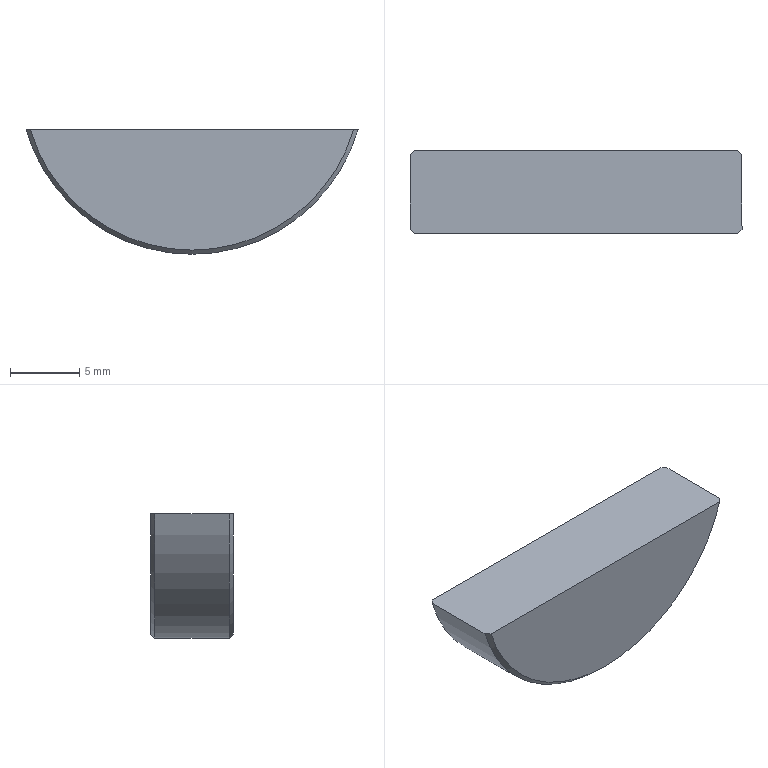Part | SolidWorks | features Chamfer 1, Extrusion 1 | 1 solid | 8 faces | box 24 x 6 x 9 mm | volume 951.697 mm3 | cone 3 | plane 3 | cylinder 2 | commonest cylinder face diameters 25 x2
STEP:
#1=CARTESIAN_POINT('',(0.,3.,-8.7));
#2=VERTEX_POINT('',#1);
#3=CARTESIAN_POINT('',(-11.687,3.,0.));
#4=VERTEX_POINT('',#3);
#5=CARTESIAN_POINT('',(0.,3.,3.5));
#6=DIRECTION('',(0.,1.,0.));
#7=DIRECTION('',(0.,0.,-1.));
#8=AXIS2_PLACEMENT_3D('',#5,#6,#7);
#9=CIRCLE('',#8,12.2);
#10=EDGE_CURVE('',#2,#4,#9,.T.);
#11=ORIENTED_EDGE('',*,*,#10,.F.);
#12=CARTESIAN_POINT('',(0.,2.7,-9.));
#13=VERTEX_POINT('',#12);
#14=CARTESIAN_POINT('',(0.,2.7,-9.));
#15=DIRECTION('',(0.,-0.7071,-0.7071));
#16=VECTOR('',#15,1000.);
#17=LINE('',#14,#16);
#18=EDGE_CURVE('',#2,#13,#17,.T.);
#19=ORIENTED_EDGE('',*,*,#18,.T.);
#20=CARTESIAN_POINT('',(-12.,2.7,0.));
#21=VERTEX_POINT('',#20);
#22=CARTESIAN_POINT('',(0.,2.7,3.5));
#23=DIRECTION('',(0.,-1.,0.));
#24=DIRECTION('',(0.,0.,-1.));
#25=AXIS2_PLACEMENT_3D('',#22,#23,#24);
#26=CIRCLE('',#25,12.5);
#27=EDGE_CURVE('',#21,#13,#26,.T.);
#28=ORIENTED_EDGE('',*,*,#27,.F.);
#29=CARTESIAN_POINT('',(-11.687,3.,0.));
#30=CARTESIAN_POINT('',(-11.792,2.9,0.));
#31=CARTESIAN_POINT('',(-11.896,2.8,0.));
#32=CARTESIAN_POINT('',(-12.,2.7,0.));
#33=B_SPLINE_CURVE_WITH_KNOTS('',3,(#29,#30,#31,#32),.UNSPECIFIED.,.F.,.F.,(4,4),(0.,0.0004334),.UNSPECIFIED.);
#34=EDGE_CURVE('',#4,#21,#33,.T.);
#35=ORIENTED_EDGE('',*,*,#34,.F.);
#36=EDGE_LOOP('',(#11,#19,#28,#35));
#37=FACE_OUTER_BOUND('',#36,.T.);
#38=CARTESIAN_POINT('',(0.,2.7,3.5));
#39=DIRECTION('',(0.,-1.,0.));
#40=DIRECTION('',(0.,0.,-1.));
#41=AXIS2_PLACEMENT_3D('',#38,#39,#40);
#42=CONICAL_SURFACE('',#41,12.5,0.7854);
#43=ADVANCED_FACE('',(#37),#42,.T.);
#44=ORIENTED_EDGE('',*,*,#27,.T.);
#45=CARTESIAN_POINT('',(0.,-2.7,-9.));
#46=VERTEX_POINT('',#45);
#47=CARTESIAN_POINT('',(0.,3.,-9.));
#48=DIRECTION('',(0.,-1.,0.));
#49=VECTOR('',#48,1000.);
#50=LINE('',#47,#49);
#51=EDGE_CURVE('',#13,#46,#50,.T.);
#52=ORIENTED_EDGE('',*,*,#51,.T.);
#53=CARTESIAN_POINT('',(-12.,-2.7,0.));
#54=VERTEX_POINT('',#53);
#55=CARTESIAN_POINT('',(0.,-2.7,3.5));
#56=DIRECTION('',(0.,1.,0.));
#57=DIRECTION('',(0.,0.,-1.));
#58=AXIS2_PLACEMENT_3D('',#55,#56,#57);
#59=CIRCLE('',#58,12.5);
#60=EDGE_CURVE('',#46,#54,#59,.T.);
#61=ORIENTED_EDGE('',*,*,#60,.T.);
#62=CARTESIAN_POINT('',(-12.,3.,0.));
#63=DIRECTION('',(0.,-1.,0.));
#64=VECTOR('',#63,1000.);
#65=LINE('',#62,#64);
#66=EDGE_CURVE('',#21,#54,#65,.T.);
#67=ORIENTED_EDGE('',*,*,#66,.F.);
#68=EDGE_LOOP('',(#44,#52,#61,#67));
#69=FACE_OUTER_BOUND('',#68,.T.);
#70=CARTESIAN_POINT('',(0.,3.,3.5));
#71=DIRECTION('',(0.,-1.,0.));
#72=DIRECTION('',(0.,0.,-1.));
#73=AXIS2_PLACEMENT_3D('',#70,#71,#72);
#74=CYLINDRICAL_SURFACE('',#73,12.5);
#75=ADVANCED_FACE('',(#69),#74,.T.);
#76=ORIENTED_EDGE('',*,*,#51,.F.);
#77=CARTESIAN_POINT('',(12.,2.7,0.));
#78=VERTEX_POINT('',#77);
#79=CARTESIAN_POINT('',(0.,2.7,3.5));
#80=DIRECTION('',(0.,-1.,0.));
#81=DIRECTION('',(0.,0.,-1.));
#82=AXIS2_PLACEMENT_3D('',#79,#80,#81);
#83=CIRCLE('',#82,12.5);
#84=EDGE_CURVE('',#13,#78,#83,.T.);
#85=ORIENTED_EDGE('',*,*,#84,.T.);
#86=CARTESIAN_POINT('',(12.,-2.7,0.));
#87=VERTEX_POINT('',#86);
#88=CARTESIAN_POINT('',(12.,3.,0.));
#89=DIRECTION('',(0.,-1.,0.));
#90=VECTOR('',#89,1000.);
#91=LINE('',#88,#90);
#92=EDGE_CURVE('',#78,#87,#91,.T.);
#93=ORIENTED_EDGE('',*,*,#92,.T.);
#94=CARTESIAN_POINT('',(0.,-2.7,3.5));
#95=DIRECTION('',(0.,1.,0.));
#96=DIRECTION('',(0.,0.,-1.));
#97=AXIS2_PLACEMENT_3D('',#94,#95,#96);
#98=CIRCLE('',#97,12.5);
#99=EDGE_CURVE('',#87,#46,#98,.T.);
#100=ORIENTED_EDGE('',*,*,#99,.T.);
#101=EDGE_LOOP('',(#76,#85,#93,#100));
#102=FACE_OUTER_BOUND('',#101,.T.);
#103=CARTESIAN_POINT('',(0.,3.,3.5));
#104=DIRECTION('',(0.,-1.,0.));
#105=DIRECTION('',(0.,0.,-1.));
#106=AXIS2_PLACEMENT_3D('',#103,#104,#105);
#107=CYLINDRICAL_SURFACE('',#106,12.5);
#108=ADVANCED_FACE('',(#102),#107,.T.);
#109=CARTESIAN_POINT('',(11.687,-3.,0.));
#110=VERTEX_POINT('',#109);
#111=CARTESIAN_POINT('',(-11.687,-3.,0.));
#112=VERTEX_POINT('',#111);
#113=CARTESIAN_POINT('',(12.,-3.,0.));
#114=DIRECTION('',(-1.,0.,0.));
#115=VECTOR('',#114,1000.);
#116=LINE('',#113,#115);
#117=EDGE_CURVE('',#110,#112,#116,.T.);
#118=ORIENTED_EDGE('',*,*,#117,.F.);
#119=CARTESIAN_POINT('',(11.687,-3.,0.));
#120=CARTESIAN_POINT('',(11.792,-2.9,0.));
#121=CARTESIAN_POINT('',(11.896,-2.8,0.));
#122=CARTESIAN_POINT('',(12.,-2.7,0.));
#123=B_SPLINE_CURVE_WITH_KNOTS('',3,(#119,#120,#121,#122),.UNSPECIFIED.,.F.,.F.,(4,4),(0.,0.0004334),.UNSPECIFIED.);
#124=EDGE_CURVE('',#110,#87,#123,.T.);
#125=ORIENTED_EDGE('',*,*,#124,.T.);
#126=ORIENTED_EDGE('',*,*,#92,.F.);
#127=CARTESIAN_POINT('',(11.687,3.,0.));
#128=VERTEX_POINT('',#127);
#129=CARTESIAN_POINT('',(12.,2.7,0.));
#130=CARTESIAN_POINT('',(11.896,2.8,0.));
#131=CARTESIAN_POINT('',(11.792,2.9,0.));
#132=CARTESIAN_POINT('',(11.687,3.,0.));
#133=B_SPLINE_CURVE_WITH_KNOTS('',3,(#129,#130,#131,#132),.UNSPECIFIED.,.F.,.F.,(4,4),(0.,0.0004334),.UNSPECIFIED.);
#134=EDGE_CURVE('',#78,#128,#133,.T.);
#135=ORIENTED_EDGE('',*,*,#134,.T.);
#136=CARTESIAN_POINT('',(12.,3.,0.));
#137=DIRECTION('',(-1.,0.,0.));
#138=VECTOR('',#137,1000.);
#139=LINE('',#136,#138);
#140=EDGE_CURVE('',#128,#4,#139,.T.);
#141=ORIENTED_EDGE('',*,*,#140,.T.);
#142=ORIENTED_EDGE('',*,*,#34,.T.);
#143=ORIENTED_EDGE('',*,*,#66,.T.);
#144=CARTESIAN_POINT('',(-12.,-2.7,0.));
#145=CARTESIAN_POINT('',(-11.896,-2.8,0.));
#146=CARTESIAN_POINT('',(-11.792,-2.9,0.));
#147=CARTESIAN_POINT('',(-11.687,-3.,0.));
#148=B_SPLINE_CURVE_WITH_KNOTS('',3,(#144,#145,#146,#147),.UNSPECIFIED.,.F.,.F.,(4,4),(0.,0.0004334),.UNSPECIFIED.);
#149=EDGE_CURVE('',#54,#112,#148,.T.);
#150=ORIENTED_EDGE('',*,*,#149,.T.);
#151=EDGE_LOOP('',(#118,#125,#126,#135,#141,#142,#143,#150));
#152=FACE_OUTER_BOUND('',#151,.T.);
#153=CARTESIAN_POINT('',(12.,3.,0.));
#154=DIRECTION('',(0.,0.,1.));
#155=DIRECTION('',(1.,0.,0.));
#156=AXIS2_PLACEMENT_3D('',#153,#154,#155);
#157=PLANE('',#156);
#158=ADVANCED_FACE('',(#152),#157,.T.);
#159=ORIENTED_EDGE('',*,*,#140,.F.);
#160=CARTESIAN_POINT('',(0.,3.,3.5));
#161=DIRECTION('',(0.,1.,0.));
#162=DIRECTION('',(0.,0.,-1.));
#163=AXIS2_PLACEMENT_3D('',#160,#161,#162);
#164=CIRCLE('',#163,12.2);
#165=EDGE_CURVE('',#128,#2,#164,.T.);
#166=ORIENTED_EDGE('',*,*,#165,.T.);
#167=ORIENTED_EDGE('',*,*,#10,.T.);
#168=EDGE_LOOP('',(#159,#166,#167));
#169=FACE_OUTER_BOUND('',#168,.T.);
#170=CARTESIAN_POINT('',(0.,3.,3.5));
#171=DIRECTION('',(0.,-1.,0.));
#172=DIRECTION('',(0.,0.,-1.));
#173=AXIS2_PLACEMENT_3D('',#170,#171,#172);
#174=PLANE('',#173);
#175=ADVANCED_FACE('',(#169),#174,.F.);
#176=ORIENTED_EDGE('',*,*,#117,.T.);
#177=CARTESIAN_POINT('',(0.,-3.,3.5));
#178=DIRECTION('',(0.,-1.,0.));
#179=DIRECTION('',(0.,0.,-1.));
#180=AXIS2_PLACEMENT_3D('',#177,#178,#179);
#181=CIRCLE('',#180,12.2);
#182=EDGE_CURVE('',#112,#110,#181,.T.);
#183=ORIENTED_EDGE('',*,*,#182,.T.);
#184=EDGE_LOOP('',(#176,#183));
#185=FACE_OUTER_BOUND('',#184,.T.);
#186=CARTESIAN_POINT('',(0.,-3.,3.5));
#187=DIRECTION('',(0.,-1.,0.));
#188=DIRECTION('',(0.,0.,-1.));
#189=AXIS2_PLACEMENT_3D('',#186,#187,#188);
#190=PLANE('',#189);
#191=ADVANCED_FACE('',(#185),#190,.T.);
#192=ORIENTED_EDGE('',*,*,#149,.F.);
#193=ORIENTED_EDGE('',*,*,#60,.F.);
#194=ORIENTED_EDGE('',*,*,#99,.F.);
#195=ORIENTED_EDGE('',*,*,#124,.F.);
#196=ORIENTED_EDGE('',*,*,#182,.F.);
#197=EDGE_LOOP('',(#192,#193,#194,#195,#196));
#198=FACE_OUTER_BOUND('',#197,.T.);
#199=CARTESIAN_POINT('',(0.,-3.,3.5));
#200=DIRECTION('',(0.,1.,0.));
#201=DIRECTION('',(0.,0.,1.));
#202=AXIS2_PLACEMENT_3D('',#199,#200,#201);
#203=CONICAL_SURFACE('',#202,12.2,0.7854);
#204=ADVANCED_FACE('',(#198),#203,.T.);
#205=ORIENTED_EDGE('',*,*,#18,.F.);
#206=ORIENTED_EDGE('',*,*,#165,.F.);
#207=ORIENTED_EDGE('',*,*,#134,.F.);
#208=ORIENTED_EDGE('',*,*,#84,.F.);
#209=EDGE_LOOP('',(#205,#206,#207,#208));
#210=FACE_OUTER_BOUND('',#209,.T.);
#211=CARTESIAN_POINT('',(0.,2.7,3.5));
#212=DIRECTION('',(0.,-1.,0.));
#213=DIRECTION('',(0.,0.,-1.));
#214=AXIS2_PLACEMENT_3D('',#211,#212,#213);
#215=CONICAL_SURFACE('',#214,12.5,0.7854);
#216=ADVANCED_FACE('',(#210),#215,.T.);
#217=CLOSED_SHELL('',(#43,#75,#108,#158,#175,#191,#204,#216));
#218=MANIFOLD_SOLID_BREP('',#217);
#219=CARTESIAN_POINT('',(0.,0.,0.));
#220=DIRECTION('',(0.,0.,1.));
#221=DIRECTION('',(1.,0.,0.));
#222=AXIS2_PLACEMENT_3D('',#219,#220,#221);
#223=(LENGTH_UNIT()NAMED_UNIT(*)SI_UNIT(.MILLI.,.METRE.));
#224=UNCERTAINTY_MEASURE_WITH_UNIT(LENGTH_MEASURE(0.00001),#223,'','');
#225=(NAMED_UNIT(*)PLANE_ANGLE_UNIT()SI_UNIT($,.RADIAN.));
#226=(NAMED_UNIT(*)SI_UNIT($,.STERADIAN.)SOLID_ANGLE_UNIT());
#227=(GEOMETRIC_REPRESENTATION_CONTEXT(3)GLOBAL_UNCERTAINTY_ASSIGNED_CONTEXT((#224))GLOBAL_UNIT_ASSIGNED_CONTEXT((#223,#225,#226))REPRESENTATION_CONTEXT('',''));
#228=ADVANCED_BREP_SHAPE_REPRESENTATION('',(#218,#222),#227);